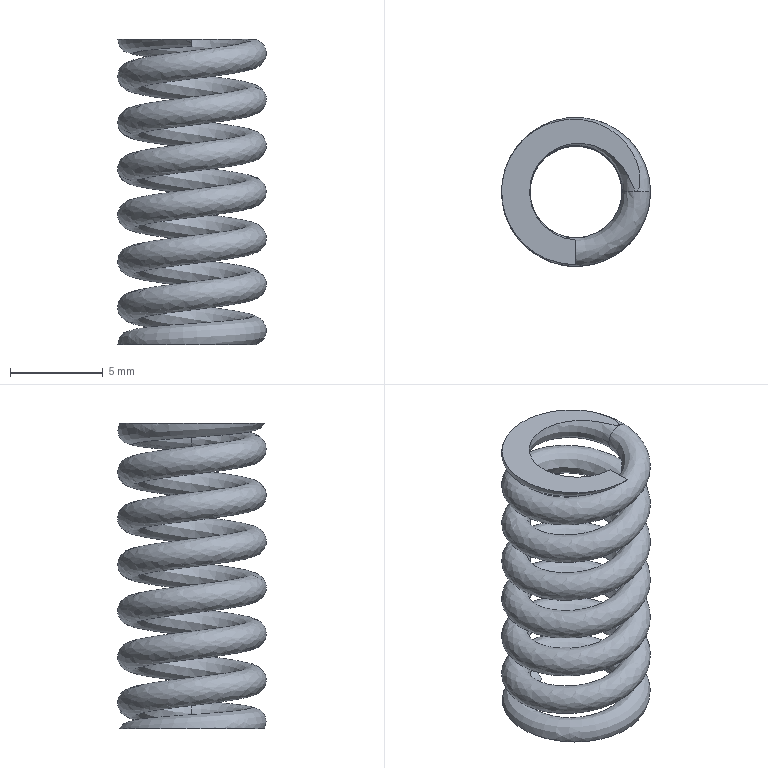Part | STEP file | Spring | 1 solid | 7 faces | volume 251.261 mm3 | plane 4 | spline 3